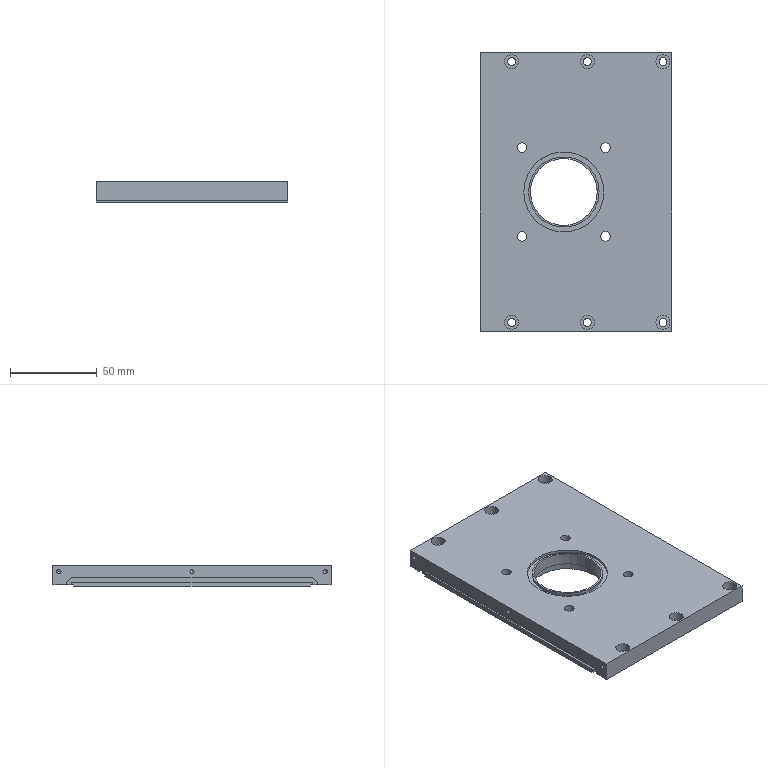NC program | NX | posted with a generic post | part box 110 x 160 x 12 mm
Whole program:
N10 G17 G21 G94 G90
(HOLE_MILLING_1 , TOOL : D4)
N12 T11 M6
N14 G54
N16 G17 G0 G90 X-75. Y37. B0. C0. S9500 M3
N18 G43 Z30. H11
N20 Z0.5
N22 G94 G3 X-76. Y36. R1. F1650.
N24 X-75. Y35. R1.
N26 X-75. Y35. Z0.1 I0. J2.
N28 X-75. Y35. Z-0.3 I0. J2.
N30 X-75. Y35. Z-0.7 I0. J2.
N32 X-75. Y35. Z-1.1 I0. J2.
N34 X-75. Y35. Z-1.5 I0. J2.
N36 X-75. Y35. Z-1.9 I0. J2.
N38 X-75. Y35. Z-2.3 I0. J2.
N40 X-75. Y35. Z-2.7 I0. J2.
N42 X-75. Y35. Z-3.1 I0. J2.
N44 X-75. Y35. Z-3.5 I0. J2.
N46 X-75. Y35. Z-3.9 I0. J2.
N48 X-75. Y35. Z-4.3 I0. J2.
N50 X-75. Y35. Z-4.7 I0. J2.
N52 X-77. Y37. Z-5. R-2.
N54 X-75. Y35. R2.
N56 X-77. Y37. R-2.
N58 X-76. Y36. R1.
N60 X-75. Y37. R1.
N62 G0 Z30.
N64 Y-6.5
N66 Z0.5
N68 G3 X-76. Y-7.5 R1.
N70 X-75. Y-8.5 R1.
N72 X-75. Y-8.5 Z0.1 I0. J2.
N74 X-75. Y-8.5 Z-0.3 I0. J2.
N76 X-75. Y-8.5 Z-0.7 I0. J2.
N78 X-75. Y-8.5 Z-1.1 I0. J2.
N80 X-75. Y-8.5 Z-1.5 I0. J2.
N82 X-75. Y-8.5 Z-1.9 I0. J2.
N84 X-75. Y-8.5 Z-2.3 I0. J2.
N86 X-75. Y-8.5 Z-2.7 I0. J2.
N88 X-75. Y-8.5 Z-3.1 I0. J2.
N90 X-75. Y-8.5 Z-3.5 I0. J2.
N92 X-75. Y-8.5 Z-3.9 I0. J2.
N94 X-75. Y-8.5 Z-4.3 I0. J2.
N96 X-75. Y-8.5 Z-4.7 I0. J2.
N98 X-77. Y-6.5 Z-5. R-2.
N100 X-75. Y-8.5 R2.
N102 X-77. Y-6.5 R-2.
N104 X-76. Y-7.5 R1.
N106 X-75. Y-6.5 R1.
N108 G0 Z30.
N110 Y-50.
N112 Z0.5
N114 G3 X-76. Y-51. R1.
N116 X-75. Y-52. R1.
N118 X-75. Y-52. Z0.1 I0. J2.
N120 X-75. Y-52. Z-0.3 I0. J2.
N122 X-75. Y-52. Z-0.7 I0. J2.
N124 X-75. Y-52. Z-1.1 I0. J2.
N126 X-75. Y-52. Z-1.5 I0. J2.
N128 X-75. Y-52. Z-1.9 I0. J2.
N130 X-75. Y-52. Z-2.3 I0. J2.
N132 X-75. Y-52. Z-2.7 I0. J2.
N134 X-75. Y-52. Z-3.1 I0. J2.
N136 X-75. Y-52. Z-3.5 I0. J2.
N138 X-75. Y-52. Z-3.9 I0. J2.
N140 X-75. Y-52. Z-4.3 I0. J2.
N142 X-75. Y-52. Z-4.7 I0. J2.
N144 X-77. Y-50. Z-5. R-2.
N146 X-75. Y-52. R2.
N148 X-77. Y-50. R-2.
N150 X-76. Y-51. R1.
N152 X-75. Y-50. R1.
N154 G0 Z30.
N156 X75.
N158 Z0.5
N160 G3 X74. Y-51. R1.
N162 X75. Y-52. R1.
N164 X75. Y-52. Z0.1 I0. J2.
N166 X75. Y-52. Z-0.3 I0. J2.
N168 X75. Y-52. Z-0.7 I0. J2.
N170 X75. Y-52. Z-1.1 I0. J2.
N172 X75. Y-52. Z-1.5 I0. J2.
N174 X75. Y-52. Z-1.9 I0. J2.
N176 X75. Y-52. Z-2.3 I0. J2.
N178 X75. Y-52. Z-2.7 I0. J2.
N180 X75. Y-52. Z-3.1 I0. J2.
N182 X75. Y-52. Z-3.5 I0. J2.
N184 X75. Y-52. Z-3.9 I0. J2.
N186 X75. Y-52. Z-4.3 I0. J2.
N188 X75. Y-52. Z-4.7 I0. J2.
N190 X73. Y-50. Z-5. R-2.
N192 X75. Y-52. R2.
N194 X73. Y-50. R-2.
N196 X74. Y-51. R1.
N198 X75. Y-50. R1.
N200 G0 Z30.
N202 Y-6.5
N204 Z0.5
N206 G3 X74. Y-7.5 R1.
N208 X75. Y-8.5 R1.
N210 X75. Y-8.5 Z0.1 I0. J2.
N212 X75. Y-8.5 Z-0.3 I0. J2.
N214 X75. Y-8.5 Z-0.7 I0. J2.
N216 X75. Y-8.5 Z-1.1 I0. J2.
N218 X75. Y-8.5 Z-1.5 I0. J2.
N220 X75. Y-8.5 Z-1.9 I0. J2.
N222 X75. Y-8.5 Z-2.3 I0. J2.
N224 X75. Y-8.5 Z-2.7 I0. J2.
N226 X75. Y-8.5 Z-3.1 I0. J2.
N228 X75. Y-8.5 Z-3.5 I0. J2.
N230 X75. Y-8.5 Z-3.9 I0. J2.
N232 X75. Y-8.5 Z-4.3 I0. J2.
N234 X75. Y-8.5 Z-4.7 I0. J2.
N236 X73. Y-6.5 Z-5. R-2.
N238 X75. Y-8.5 R2.
N240 X73. Y-6.5 R-2.
N242 X74. Y-7.5 R1.
N244 X75. Y-6.5 R1.
N246 G0 Z30.
N248 Y37.
N250 Z0.5
N252 G3 X74. Y36. R1.
N254 X75. Y35. R1.
N256 X75. Y35. Z0.1 I0. J2.
N258 X75. Y35. Z-0.3 I0. J2.
N260 X75. Y35. Z-0.7 I0. J2.
N262 X75. Y35. Z-1.1 I0. J2.
N264 X75. Y35. Z-1.5 I0. J2.
N266 X75. Y35. Z-1.9 I0. J2.
N268 X75. Y35. Z-2.3 I0. J2.
N270 X75. Y35. Z-2.7 I0. J2.
N272 X75. Y35. Z-3.1 I0. J2.
N274 X75. Y35. Z-3.5 I0. J2.
N276 X75. Y35. Z-3.9 I0. J2.
N278 X75. Y35. Z-4.3 I0. J2.
N280 X75. Y35. Z-4.7 I0. J2.
N282 X73. Y37. Z-5. R-2.
N284 X75. Y35. R2.
N286 X73. Y37. R-2.
N288 X74. Y36. R1.
N290 X75. Y37. R1.
N292 G0 Z30.
N294 M5
(ZLEVEL_PROFILE , TOOL : D2)
N296 T02 M6
N298 G54
N300 G17 G0 G90 X19.994 Y-2.325 B0. C0. S9500 M3
N302 G43 Z30. H2
N304 Z1.
N306 G94 G1 X20.195 Y-1.926 Z0.977 F1100.
N308 X21.236 Y0.952 Z0.816
N310 X21.868 Y3.947 Z0.656
N312 X22.08 Y7. Z0.495
N314 X21.868 Y10.053 Z0.335
N316 X21.236 Y13.048 Z0.175
N318 X20.195 Y15.926 Z0.014
N320 X19.676 Y16.953 Z-0.046
N322 X19.653 Y16.999 Z-0.049
N324 X19.215 Y17.859 Z-0.099
N326 X18.703 Y18.678 Z-0.15
N328 G3 X-19.653 Y16.999 R22.05
N330 G1 X-19.676 Y16.953
N332 G3 X-9.953 Y-12.676 R22.05
N334 X19.653 Y-2.999 R22.05
N336 G1 X19.676 Y-2.953
N338 G3 X19.676 Y16.953 R22.05
N340 G1 X19.653 Y16.999
N342 G3 X18.703 Y18.678 R22.05
N344 G1 X18.604 Y18.819 Z-0.153
N346 X18.506 Y18.96 Z-0.156
N348 X18.408 Y19.101 Z-0.159
N350 X18.31 Y19.242 Z-0.162
N352 X18.212 Y19.383 Z-0.165
N354 X18.114 Y19.524 Z-0.168
N356 X18.016 Y19.665 Z-0.171
N358 X17.917 Y19.806 Z-0.174
N360 X17.819 Y19.947 Z-0.177
N362 X17.722 Y20.088 Z-0.18
N364 X17.623 Y20.229 Z-0.183
N366 X17.525 Y20.37 Z-0.186
N368 X17.426 Y20.51 Z-0.189
N370 X17.314 Y20.64 Z-0.192
N372 X17.201 Y20.771 Z-0.195
N374 X17.089 Y20.901 Z-0.198
N376 X16.978 Y21.031 Z-0.201
N378 X16.866 Y21.162 Z-0.204
N380 X16.754 Y21.292 Z-0.207
N382 X16.642 Y21.422 Z-0.21
N384 X16.53 Y21.552 Z-0.213
N386 X16.418 Y21.682 Z-0.216
N388 X16.306 Y21.813 Z-0.219
N390 X16.195 Y21.943 Z-0.222
N392 X16.082 Y22.074 Z-0.225
N394 X15.97 Y22.204 Z-0.228
N396 X15.845 Y22.322 Z-0.231
N398 X15.72 Y22.44 Z-0.234
N400 X15.595 Y22.558 Z-0.237
N402 X15.471 Y22.677 Z-0.24
N404 X15.346 Y22.795 Z-0.243
N406 X15.222 Y22.913 Z-0.246
N408 X15.098 Y23.031 Z-0.249
N410 X14.973 Y23.15 Z-0.252
N412 X14.849 Y23.268 Z-0.255
N414 X14.725 Y23.387 Z-0.258
N416 X14.6 Y23.505 Z-0.261
N418 X14.475 Y23.623 Z-0.264
N420 X14.35 Y23.741 Z-0.267
N422 X14.214 Y23.846 Z-0.27
N424 X14.078 Y23.951 Z-0.273
N426 X13.942 Y24.056 Z-0.276
N428 X13.806 Y24.161 Z-0.279
N430 X13.67 Y24.267 Z-0.282
N432 X13.534 Y24.371 Z-0.285
N434 X13.399 Y24.476 Z-0.288
N436 X13.263 Y24.581 Z-0.291
N438 X13.127 Y24.686 Z-0.294
N440 X12.991 Y24.792 Z-0.297
N442 X12.864 Y24.909 Z-0.3
N444 G3 X-19.653 Y16.999 R22.05
N446 G1 X-19.676 Y16.953
N448 G3 X-9.953 Y-12.676 R22.05
N450 X19.653 Y-2.999 R22.05
N452 G1 X19.676 Y-2.953
N454 G3 X19.676 Y16.953 R22.05
N456 G1 X19.653 Y16.999
N458 G3 X18.703 Y18.678 R22.05
N460 G1 X18.605 Y18.819 Z-0.303
N462 X18.506 Y18.96 Z-0.306
N464 X18.408 Y19.101 Z-0.309
N466 X18.31 Y19.242 Z-0.312
N468 X18.211 Y19.383 Z-0.315
N470 X18.114 Y19.524 Z-0.318
N472 X18.015 Y19.664 Z-0.321
N474 X17.917 Y19.805 Z-0.324
N476 X17.819 Y19.946 Z-0.327
N478 X17.722 Y20.088 Z-0.33
N480 X17.623 Y20.228 Z-0.333
N482 X17.525 Y20.37 Z-0.336
N484 X17.426 Y20.51 Z-0.339
N486 X17.313 Y20.64 Z-0.342
N488 X17.201 Y20.77 Z-0.345
N490 X17.089 Y20.901 Z-0.348
N492 X16.977 Y21.031 Z-0.351
N494 X16.866 Y21.162 Z-0.354
N496 X16.754 Y21.292 Z-0.357
N498 X16.642 Y21.422 Z-0.36
N500 X16.53 Y21.552 Z-0.363
N502 X16.418 Y21.682 Z-0.366
N504 X16.306 Y21.813 Z-0.369
N506 X16.195 Y21.943 Z-0.372
N508 X16.083 Y22.074 Z-0.375
N510 X15.97 Y22.204 Z-0.378
N512 X15.845 Y22.322 Z-0.381
N514 X15.72 Y22.44 Z-0.384
N516 X15.596 Y22.559 Z-0.387
N518 X15.471 Y22.676 Z-0.39
N520 X15.347 Y22.795 Z-0.393
N522 X15.222 Y22.913 Z-0.396
N524 X15.097 Y23.031 Z-0.399
N526 X14.973 Y23.15 Z-0.402
N528 X14.849 Y23.268 Z-0.405
N530 X14.725 Y23.387 Z-0.408
N532 X14.6 Y23.505 Z-0.411
N534 X14.475 Y23.623 Z-0.414
N536 X14.35 Y23.741 Z-0.417
N538 X14.214 Y23.846 Z-0.42
N540 X14.077 Y23.951 Z-0.423
N542 X13.942 Y24.056 Z-0.426
N544 X13.806 Y24.161 Z-0.429
N546 X13.67 Y24.266 Z-0.432
N548 X13.534 Y24.371 Z-0.435
N550 X13.399 Y24.476 Z-0.438
N552 X13.263 Y24.582 Z-0.441
N554 X13.127 Y24.686 Z-0.444
N556 X12.991 Y24.792 Z-0.447
N558 X12.864 Y24.909 Z-0.45
N560 G3 X-19.653 Y16.999 R22.05
N562 G1 X-19.676 Y16.953
N564 G3 X-9.953 Y-12.676 R22.05
N566 X19.653 Y-2.999 R22.05
N568 G1 X19.676 Y-2.953
N570 G3 X19.676 Y16.953 R22.05
N572 G1 X19.653 Y16.999
N574 G3 X18.703 Y18.678 R22.05
N576 G1 X18.604 Y18.819 Z-0.453
N578 X18.506 Y18.96 Z-0.456
N580 X18.408 Y19.101 Z-0.459
N582 X18.309 Y19.242 Z-0.462
N584 X18.212 Y19.383 Z-0.465
N586 X18.114 Y19.524 Z-0.468
N588 X18.016 Y19.665 Z-0.471
N590 X17.917 Y19.805 Z-0.474
N592 X17.819 Y19.946 Z-0.477
N594 X17.721 Y20.087 Z-0.48
N596 X17.623 Y20.228 Z-0.483
N598 X17.525 Y20.37 Z-0.486
N600 X17.426 Y20.51 Z-0.489
N602 X17.313 Y20.64 Z-0.492
N604 X17.201 Y20.77 Z-0.495
N606 X17.089 Y20.901 Z-0.498
N608 X16.978 Y21.031 Z-0.501
N610 X16.866 Y21.162 Z-0.504
N612 X16.753 Y21.291 Z-0.507
N614 X16.642 Y21.422 Z-0.51
N616 X16.53 Y21.552 Z-0.513
N618 X16.418 Y21.682 Z-0.516
N620 X16.307 Y21.813 Z-0.519
N622 X16.195 Y21.943 Z-0.522
N624 X16.083 Y22.074 Z-0.525
N626 X15.97 Y22.204 Z-0.528
N628 X15.845 Y22.321 Z-0.531
N630 X15.72 Y22.44 Z-0.534
N632 X15.595 Y22.558 Z-0.537
N634 X15.471 Y22.676 Z-0.54
N636 X15.347 Y22.795 Z-0.543
N638 X15.222 Y22.913 Z-0.546
N640 X15.098 Y23.031 Z-0.549
N642 X14.973 Y23.149 Z-0.552
N644 X14.849 Y23.268 Z-0.555
N646 X14.724 Y23.386 Z-0.558
N648 X14.599 Y23.504 Z-0.561
N650 X14.475 Y23.623 Z-0.564
N652 X14.35 Y23.741 Z-0.567
N654 X14.213 Y23.846 Z-0.57
N656 X14.078 Y23.951 Z-0.573
N658 X13.941 Y24.056 Z-0.576
N660 X13.806 Y24.161 Z-0.579
N662 X13.67 Y24.266 Z-0.582
N664 X13.534 Y24.371 Z-0.585
N666 X13.398 Y24.476 Z-0.588
N668 X13.263 Y24.581 Z-0.591
N670 X13.127 Y24.686 Z-0.594
N672 X12.991 Y24.791 Z-0.597
N674 X12.864 Y24.909 Z-0.6
N676 G3 X-19.653 Y16.999 R22.05
N678 G1 X-19.676 Y16.953
N680 G3 X-9.953 Y-12.676 R22.05
N682 X19.653 Y-2.999 R22.05
N684 G1 X19.676 Y-2.953
N686 G3 X19.676 Y16.953 R22.05
N688 G1 X19.653 Y16.999
N690 G3 X18.703 Y18.678 R22.05
N692 G1 X18.604 Y18.819 Z-0.603
N694 X18.506 Y18.96 Z-0.606
N696 X18.408 Y19.101 Z-0.609
N698 X18.309 Y19.242 Z-0.612
N700 X18.211 Y19.383 Z-0.615
N702 X18.113 Y19.524 Z-0.618
N704 X18.015 Y19.665 Z-0.621
N706 X17.917 Y19.805 Z-0.624
N708 X17.819 Y19.946 Z-0.627
N710 X17.721 Y20.087 Z-0.63
N712 X17.622 Y20.228 Z-0.633
N714 X17.525 Y20.369 Z-0.636
N716 X17.426 Y20.51 Z-0.639
N718 X17.313 Y20.64 Z-0.642
N720 X17.201 Y20.77 Z-0.645
N722 X17.089 Y20.901 Z-0.648
N724 X16.977 Y21.031 Z-0.651
N726 X16.866 Y21.161 Z-0.654
N728 X16.754 Y21.292 Z-0.657
N730 X16.642 Y21.422 Z-0.66
N732 X16.53 Y21.552 Z-0.663
N734 X16.418 Y21.682 Z-0.666
N736 X16.306 Y21.813 Z-0.669
N738 X16.194 Y21.943 Z-0.672
N740 X16.082 Y22.074 Z-0.675
N742 X15.97 Y22.204 Z-0.678
N744 X15.844 Y22.321 Z-0.681
N746 X15.72 Y22.44 Z-0.684
N748 X15.595 Y22.558 Z-0.687
N750 X15.471 Y22.676 Z-0.69
N752 X15.346 Y22.795 Z-0.693
N754 X15.222 Y22.913 Z-0.696
N756 X15.098 Y23.031 Z-0.699
N758 X14.973 Y23.149 Z-0.702
N760 X14.849 Y23.268 Z-0.705
N762 X14.724 Y23.386 Z-0.708
N764 X14.6 Y23.505 Z-0.711
N766 X14.475 Y23.623 Z-0.714
N768 X14.35 Y23.741 Z-0.717
N770 X14.213 Y23.846 Z-0.72
N772 X14.077 Y23.951 Z-0.723
N774 X13.941 Y24.056 Z-0.726
N776 X13.806 Y24.161 Z-0.729
N778 X13.67 Y24.266 Z-0.732
N780 X13.534 Y24.371 Z-0.735
N782 X13.398 Y24.476 Z-0.738
N784 X13.263 Y24.581 Z-0.741
N786 X13.127 Y24.686 Z-0.744
N788 X12.991 Y24.791 Z-0.747
N790 X12.864 Y24.909 Z-0.75
N792 G3 X-19.653 Y16.999 R22.05
N794 G1 X-19.676 Y16.953
N796 G3 X-9.953 Y-12.676 R22.05
N798 X19.653 Y-2.999 R22.05
N800 G1 X19.676 Y-2.953
N802 G3 X19.676 Y16.953 R22.05
N804 G1 X19.653 Y16.999
N806 G3 X18.703 Y18.678 R22.05
N808 G1 X18.604 Y18.819 Z-0.753
N810 X18.506 Y18.96 Z-0.756
N812 X18.407 Y19.101 Z-0.759
N814 X18.309 Y19.242 Z-0.762
N816 X18.211 Y19.382 Z-0.765
N818 X18.113 Y19.523 Z-0.768
N820 X18.015 Y19.664 Z-0.771
N822 X17.917 Y19.805 Z-0.774
N824 X17.819 Y19.946 Z-0.777
N826 X17.721 Y20.087 Z-0.78
N828 X17.623 Y20.228 Z-0.783
N830 X17.525 Y20.369 Z-0.786
N832 X17.426 Y20.51 Z-0.789
N834 X17.313 Y20.64 Z-0.792
N836 X17.201 Y20.77 Z-0.795
N838 X17.089 Y20.901 Z-0.798
N840 X16.977 Y21.031 Z-0.801
N842 X16.865 Y21.161 Z-0.804
N844 X16.753 Y21.291 Z-0.807
N846 X16.642 Y21.422 Z-0.81
N848 X16.53 Y21.552 Z-0.813
N850 X16.418 Y21.682 Z-0.816
N852 X16.306 Y21.812 Z-0.819
N854 X16.194 Y21.943 Z-0.822
N856 X16.082 Y22.073 Z-0.825
N858 X15.97 Y22.204 Z-0.828
N860 X15.844 Y22.321 Z-0.831
N862 X15.72 Y22.44 Z-0.834
N864 X15.595 Y22.558 Z-0.837
N866 X15.47 Y22.676 Z-0.84
N868 X15.346 Y22.794 Z-0.843
N870 X15.222 Y22.913 Z-0.846
N872 X15.097 Y23.031 Z-0.849
N874 X14.973 Y23.149 Z-0.852
N876 X14.848 Y23.268 Z-0.855
N878 X14.724 Y23.386 Z-0.858
N880 X14.6 Y23.504 Z-0.861
N882 X14.475 Y23.623 Z-0.864
N884 X14.35 Y23.741 Z-0.867
N886 X14.213 Y23.845 Z-0.87
N888 X14.077 Y23.95 Z-0.873
N890 X13.941 Y24.056 Z-0.876
N892 X13.805 Y24.161 Z-0.879
N894 X13.67 Y24.266 Z-0.882
N896 X13.534 Y24.371 Z-0.885
N898 X13.398 Y24.476 Z-0.888
N900 X13.262 Y24.581 Z-0.891
N902 X13.127 Y24.686 Z-0.894
N904 X12.991 Y24.791 Z-0.897
N906 X12.864 Y24.909 Z-0.9
N908 G3 X-19.653 Y16.999 R22.05
N910 G1 X-19.676 Y16.953
N912 G3 X-9.953 Y-12.676 R22.05
N914 X19.653 Y-2.999 R22.05
N916 G1 X19.676 Y-2.953
N918 G3 X19.676 Y16.953 R22.05
N920 G1 X19.653 Y16.999
N922 G3 X18.703 Y18.678 R22.05
N924 G1 X18.604 Y18.818 Z-0.903
N926 X18.506 Y18.96 Z-0.906
N928 X18.407 Y19.1 Z-0.909
N930 X18.309 Y19.241 Z-0.912
N932 X18.211 Y19.382 Z-0.915
N934 X18.113 Y19.523 Z-0.918
N936 X18.015 Y19.664 Z-0.921
N938 X17.917 Y19.805 Z-0.924
N940 X17.819 Y19.946 Z-0.927
N942 X17.721 Y20.087 Z-0.93
N944 X17.623 Y20.228 Z-0.933
N946 X17.524 Y20.369 Z-0.936
N948 X17.426 Y20.51 Z-0.939
N950 X17.313 Y20.64 Z-0.942
N952 X17.201 Y20.77 Z-0.945
N954 X17.089 Y20.9 Z-0.948
N956 X16.977 Y21.031 Z-0.951
N958 X16.865 Y21.161 Z-0.954
N960 X16.753 Y21.291 Z-0.957
N962 X16.641 Y21.422 Z-0.96
N964 X16.529 Y21.552 Z-0.963
N966 X16.418 Y21.682 Z-0.966
N968 X16.306 Y21.812 Z-0.969
N970 X16.194 Y21.943 Z-0.972
N972 X16.082 Y22.073 Z-0.975
N974 X15.97 Y22.204 Z-0.978
N976 X15.844 Y22.321 Z-0.981
N978 X15.72 Y22.44 Z-0.984
N980 X15.595 Y22.558 Z-0.987
N982 X15.47 Y22.676 Z-0.99
N984 X15.346 Y22.794 Z-0.993
N986 X15.222 Y22.913 Z-0.996
N988 X15.097 Y23.031 Z-0.999
N990 X14.973 Y23.149 Z-1.002
N992 X14.848 Y23.267 Z-1.005
N994 X14.724 Y23.386 Z-1.008
N996 X14.599 Y23.504 Z-1.011
N998 X14.475 Y23.623 Z-1.014
N1000 X14.35 Y23.741 Z-1.017
N1002 X14.213 Y23.845 Z-1.02
N1004 X14.077 Y23.95 Z-1.023
N1006 X13.941 Y24.055 Z-1.026
N1008 X13.805 Y24.16 Z-1.029
N1010 X13.67 Y24.266 Z-1.032
N1012 X13.534 Y24.371 Z-1.035
N1014 X13.398 Y24.476 Z-1.038
N1016 X13.262 Y24.581 Z-1.041
N1018 X13.127 Y24.686 Z-1.044
N1020 X12.991 Y24.791 Z-1.047
N1022 X12.864 Y24.909 Z-1.05
N1024 G3 X-19.653 Y16.999 R22.05
N1026 G1 X-19.676 Y16.953
N1028 G3 X-9.953 Y-12.676 R22.05
N1030 X19.653 Y-2.999 R22.05
N1032 G1 X19.676 Y-2.953
N1034 G3 X19.676 Y16.953 R22.05
N1036 G1 X19.653 Y16.999
N1038 G3 X18.703 Y18.678 R22.05
N1040 G1 X18.603 Y18.818 Z-1.053
N1042 X18.505 Y18.96 Z-1.056
N1044 X18.407 Y19.1 Z-1.059
N1046 X18.309 Y19.241 Z-1.062
N1048 X18.211 Y19.382 Z-1.065
N1050 X18.113 Y19.523 Z-1.068
N1052 X18.015 Y19.664 Z-1.071
N1054 X17.917 Y19.805 Z-1.074
N1056 X17.818 Y19.946 Z-1.077
N1058 X17.721 Y20.087 Z-1.08
N1060 X17.622 Y20.228 Z-1.083
N1062 X17.524 Y20.369 Z-1.086
N1064 X17.426 Y20.51 Z-1.089
N1066 X17.313 Y20.64 Z-1.092
N1068 X17.2 Y20.77 Z-1.095
N1070 X17.089 Y20.9 Z-1.098
N1072 X16.977 Y21.03 Z-1.101
N1074 X16.865 Y21.161 Z-1.104
N1076 X16.753 Y21.291 Z-1.107
N1078 X16.641 Y21.421 Z-1.11
N1080 X16.53 Y21.552 Z-1.113
N1082 X16.418 Y21.682 Z-1.116
N1084 X16.306 Y21.812 Z-1.119
N1086 X16.194 Y21.943 Z-1.122
N1088 X16.082 Y22.073 Z-1.125
N1090 X15.97 Y22.204 Z-1.128
N1092 X15.844 Y22.321 Z-1.131
N1094 X15.719 Y22.439 Z-1.134
N1096 X15.595 Y22.558 Z-1.137
N1098 X15.47 Y22.676 Z-1.14
N1100 X15.346 Y22.795 Z-1.143
N1102 X15.222 Y22.913 Z-1.146
N1104 X15.097 Y23.031 Z-1.149
N1106 X14.973 Y23.149 Z-1.152
N1108 X14.848 Y23.267 Z-1.155
N1110 X14.724 Y23.386 Z-1.158
N1112 X14.599 Y23.504 Z-1.161
N1114 X14.475 Y23.623 Z-1.164
N1116 X14.35 Y23.741 Z-1.167
N1118 X14.213 Y23.845 Z-1.17
N1120 X14.077 Y23.95 Z-1.173
N1122 X13.941 Y24.055 Z-1.176
N1124 X13.805 Y24.16 Z-1.179
N1126 X13.67 Y24.266 Z-1.182
N1128 X13.534 Y24.37 Z-1.185
N1130 X13.398 Y24.476 Z-1.188
N1132 X13.262 Y24.581 Z-1.191
N1134 X13.126 Y24.686 Z-1.194
N1136 X12.991 Y24.791 Z-1.197
N1138 X12.864 Y24.909 Z-1.2
N1140 G3 X-19.653 Y16.999 R22.05
N1142 G1 X-19.676 Y16.953
N1144 G3 X-9.953 Y-12.676 R22.05
N1146 X19.653 Y-2.999 R22.05
N1148 G1 X19.676 Y-2.953
N1150 G3 X19.676 Y16.953 R22.05
N1152 G1 X19.653 Y16.999
N1154 G3 X18.703 Y18.678 R22.05
N1156 G1 X18.603 Y18.818 Z-1.203
N1158 X18.505 Y18.959 Z-1.206
N1160 X18.407 Y19.101 Z-1.209
N1162 X18.309 Y19.241 Z-1.212
N1164 X18.211 Y19.382 Z-1.215
N1166 X18.113 Y19.523 Z-1.218
N1168 X18.015 Y19.664 Z-1.221
N1170 X17.917 Y19.805 Z-1.224
N1172 X17.818 Y19.946 Z-1.227
N1174 X17.721 Y20.087 Z-1.23
N1176 X17.622 Y20.228 Z-1.233
N1178 X17.524 Y20.369 Z-1.236
N1180 X17.426 Y20.51 Z-1.239
N1182 X17.313 Y20.64 Z-1.242
N1184 X17.2 Y20.77 Z-1.245
N1186 X17.088 Y20.9 Z-1.248
N1188 X16.977 Y21.031 Z-1.251
N1190 X16.865 Y21.161 Z-1.254
N1192 X16.753 Y21.291 Z-1.257
N1194 X16.641 Y21.421 Z-1.26
N1196 X16.529 Y21.552 Z-1.263
N1198 X16.417 Y21.682 Z-1.266
N1200 X16.306 Y21.812 Z-1.269
N1202 X16.194 Y21.943 Z-1.272
N1204 X16.082 Y22.073 Z-1.275
N1206 X15.97 Y22.204 Z-1.278
N1208 X15.844 Y22.321 Z-1.281
N1210 X15.719 Y22.439 Z-1.284
N1212 X15.595 Y22.558 Z-1.287
N1214 X15.47 Y22.676 Z-1.29
N1216 X15.346 Y22.794 Z-1.293
N1218 X15.221 Y22.912 Z-1.296
N1220 X15.097 Y23.031 Z-1.299
N1222 X14.973 Y23.149 Z-1.302
N1224 X14.848 Y23.267 Z-1.305
N1226 X14.724 Y23.386 Z-1.308
N1228 X14.599 Y23.504 Z-1.311
N1230 X14.475 Y23.622 Z-1.314
N1232 X14.35 Y23.741 Z-1.317
N1234 X14.213 Y23.845 Z-1.32
N1236 X14.077 Y23.95 Z-1.323
N1238 X13.941 Y24.055 Z-1.326
N1240 X13.805 Y24.161 Z-1.329
N1242 X13.67 Y24.266 Z-1.332
N1244 X13.534 Y24.371 Z-1.335
N1246 X13.398 Y24.476 Z-1.338
N1248 X13.262 Y24.581 Z-1.341
N1250 X13.126 Y24.686 Z-1.344
N1252 X12.991 Y24.791 Z-1.347
N1254 X12.864 Y24.909 Z-1.35
N1256 G3 X-19.653 Y16.999 R22.05
N1258 G1 X-19.676 Y16.953
N1260 G3 X-9.953 Y-12.676 R22.05
N1262 X19.653 Y-2.999 R22.05
N1264 G1 X19.676 Y-2.953
N1266 G3 X19.676 Y16.953 R22.05
N1268 G1 X19.653 Y16.999
N1270 G3 X18.703 Y18.678 R22.05
N1272 G1 X18.603 Y18.818 Z-1.353
N1274 X18.505 Y18.959 Z-1.356
N1276 X18.407 Y19.1 Z-1.359
N1278 X18.309 Y19.241 Z-1.362
N1280 X18.211 Y19.382 Z-1.365
N1282 X18.113 Y19.523 Z-1.368
N1284 X18.015 Y19.664 Z-1.371
N1286 X17.916 Y19.805 Z-1.374
N1288 X17.819 Y19.946 Z-1.377
N1290 X17.721 Y20.087 Z-1.38
N1292 X17.622 Y20.227 Z-1.383
N1294 X17.524 Y20.369 Z-1.386
N1296 X17.426 Y20.51 Z-1.389
N1298 X17.312 Y20.64 Z-1.392
N1300 X17.2 Y20.77 Z-1.395
N1302 X17.088 Y20.9 Z-1.398
N1304 X16.977 Y21.031 Z-1.401
N1306 X16.865 Y21.161 Z-1.404
N1308 X16.753 Y21.291 Z-1.407
N1310 X16.641 Y21.421 Z-1.41
N1312 X16.529 Y21.551 Z-1.413
N1314 X16.417 Y21.682 Z-1.416
N1316 X16.306 Y21.812 Z-1.419
N1318 X16.194 Y21.943 Z-1.422
N1320 X16.081 Y22.073 Z-1.425
N1322 X15.97 Y22.204 Z-1.428
N1324 X15.844 Y22.32 Z-1.431
N1326 X15.719 Y22.439 Z-1.434
N1328 X15.595 Y22.557 Z-1.437
N1330 X15.47 Y22.676 Z-1.44
N1332 X15.346 Y22.794 Z-1.443
N1334 X15.221 Y22.912 Z-1.446
N1336 X15.097 Y23.031 Z-1.449
N1338 X14.972 Y23.149 Z-1.452
N1340 X14.848 Y23.267 Z-1.455
N1342 X14.724 Y23.386 Z-1.458
N1344 X14.599 Y23.504 Z-1.461
N1346 X14.475 Y23.622 Z-1.464
N1348 X14.35 Y23.741 Z-1.467
N1350 X14.213 Y23.845 Z-1.47
N1352 X14.077 Y23.95 Z-1.473
N1354 X13.941 Y24.055 Z-1.476
N1356 X13.805 Y24.16 Z-1.479
N1358 X13.669 Y24.265 Z-1.482
N1360 X13.534 Y24.37 Z-1.485
N1362 X13.398 Y24.475 Z-1.488
N1364 X13.262 Y24.58 Z-1.491
N1366 X13.126 Y24.685 Z-1.494
N1368 X12.991 Y24.791 Z-1.497
N1370 X12.864 Y24.909 Z-1.5
N1372 G3 X-19.653 Y16.999 R22.05
N1374 G1 X-19.676 Y16.953
N1376 G3 X-9.953 Y-12.676 R22.05
N1378 X19.653 Y-2.999 R22.05
N1380 G1 X19.676 Y-2.953
N1382 G3 X19.676 Y16.953 R22.05
N1384 G1 X19.653 Y16.999
N1386 G3 X12.864 Y24.909 R22.05
N1388 G1 Z-0.5
N1390 G0 Z30.
N1392 X-18.252 Y17.909
N1394 Z1.
N1396 G1 X-16.601 Y20.314 Z0.847
N1398 X-14.454 Y22.618 Z0.682
N1400 X-11.992 Y24.579 Z0.517
N1402 X-10.061 Y25.752 Z0.399
N1404 X-7.217 Y27.019 Z0.236
N1406 X-4.218 Y27.858 Z0.072
N1408 X-1.13 Y28.25 Z-0.091
N1410 X0. Z-0.15
N1412 G2 X21.25 Y7. R21.25
N1414 X0. Y28.25 R-21.25
N1416 G1 X0.172 Y28.249 Z-0.153
N1418 X0.344 Y28.247 Z-0.156
N1420 X0.516 Y28.244 Z-0.159
N1422 X0.687 Y28.239 Z-0.162
N1424 X0.859 Y28.233 Z-0.165
N1426 X1.031 Y28.225 Z-0.168
N1428 X1.202 Y28.216 Z-0.171
N1430 X1.374 Y28.206 Z-0.174
N1432 X1.545 Y28.194 Z-0.177
N1434 X1.717 Y28.181 Z-0.18
N1436 X1.888 Y28.166 Z-0.183
N1438 X2.059 Y28.15 Z-0.186
N1440 X2.23 Y28.133 Z-0.189
N1442 X2.401 Y28.114 Z-0.192
N1444 X2.572 Y28.094 Z-0.195
N1446 X2.742 Y28.072 Z-0.198
N1448 X2.913 Y28.049 Z-0.201
N1450 X3.083 Y28.025 Z-0.204
N1452 X3.253 Y28. Z-0.207
N1454 X3.422 Y27.973 Z-0.21
N1456 X3.592 Y27.944 Z-0.213
N1458 X3.761 Y27.914 Z-0.216
N1460 X3.93 Y27.883 Z-0.219
N1462 X4.099 Y27.851 Z-0.222
N1464 X4.268 Y27.817 Z-0.225
N1466 X4.436 Y27.782 Z-0.228
N1468 X4.604 Y27.745 Z-0.231
N1470 X4.771 Y27.707 Z-0.234
N1472 X4.939 Y27.668 Z-0.237
N1474 X5.106 Y27.628 Z-0.24
N1476 X5.272 Y27.586 Z-0.243
N1478 X5.439 Y27.542 Z-0.246
N1480 X5.605 Y27.498 Z-0.249
N1482 X5.77 Y27.452 Z-0.252
N1484 X5.935 Y27.404 Z-0.255
N1486 X6.1 Y27.356 Z-0.258
N1488 X6.265 Y27.306 Z-0.261
N1490 X6.429 Y27.254 Z-0.264
N1492 X6.592 Y27.202 Z-0.267
N1494 X6.755 Y27.148 Z-0.27
N1496 X6.918 Y27.092 Z-0.273
N1498 X7.081 Y27.036 Z-0.276
N1500 X7.242 Y26.978 Z-0.279
N1502 X7.404 Y26.919 Z-0.282
N1504 X7.565 Y26.858 Z-0.285
N1506 X7.725 Y26.796 Z-0.288
N1508 X7.885 Y26.733 Z-0.291
N1510 X8.044 Y26.669 Z-0.294
N1512 X8.203 Y26.603 Z-0.297
N1514 X8.361 Y26.536 Z-0.3
N1516 G2 X0. Y28.25 R-21.25
N1518 G1 X0.172 Y28.249 Z-0.303
N1520 X0.344 Y28.247 Z-0.306
N1522 X0.516 Y28.244 Z-0.309
N1524 X0.687 Y28.239 Z-0.312
N1526 X0.859 Y28.233 Z-0.315
N1528 X1.031 Y28.225 Z-0.318
N1530 X1.202 Y28.216 Z-0.321
N1532 X1.374 Y28.206 Z-0.324
N1534 X1.545 Y28.194 Z-0.327
N1536 X1.717 Y28.181 Z-0.33
N1538 X1.888 Y28.166 Z-0.333
N1540 X2.059 Y28.15 Z-0.336
N1542 X2.23 Y28.133 Z-0.339
N1544 X2.401 Y28.114 Z-0.342
N1546 X2.572 Y28.094 Z-0.345
N1548 X2.742 Y28.072 Z-0.348
N1550 X2.913 Y28.049 Z-0.351
N1552 X3.083 Y28.025 Z-0.354
N1554 X3.253 Y28. Z-0.357
N1556 X3.422 Y27.973 Z-0.36
N1558 X3.592 Y27.944 Z-0.363
N1560 X3.761 Y27.914 Z-0.366
N1562 X3.93 Y27.883 Z-0.369
N1564 X4.099 Y27.851 Z-0.372
N1566 X4.268 Y27.817 Z-0.375
N1568 X4.436 Y27.782 Z-0.378
N1570 X4.604 Y27.745 Z-0.381
N1572 X4.771 Y27.707 Z-0.384
N1574 X4.939 Y27.668 Z-0.387
N1576 X5.106 Y27.628 Z-0.39
N1578 X5.272 Y27.586 Z-0.393
N1580 X5.439 Y27.542 Z-0.396
N1582 X5.605 Y27.498 Z-0.399
N1584 X5.77 Y27.452 Z-0.402
N1586 X5.935 Y27.404 Z-0.405
N1588 X6.1 Y27.356 Z-0.408
N1590 X6.265 Y27.306 Z-0.411
N1592 X6.429 Y27.254 Z-0.414
N1594 X6.592 Y27.202 Z-0.417
N1596 X6.755 Y27.148 Z-0.42
N1598 X6.918 Y27.092 Z-0.423
N1600 X7.081 Y27.036 Z-0.426
N1602 X7.242 Y26.978 Z-0.429
N1604 X7.404 Y26.919 Z-0.432
N1606 X7.565 Y26.858 Z-0.435
N1608 X7.725 Y26.796 Z-0.438
N1610 X7.885 Y26.733 Z-0.441
N1612 X8.044 Y26.669 Z-0.444
N1614 X8.203 Y26.603 Z-0.447
N1616 X8.361 Y26.536 Z-0.45
N1618 G2 X0. Y28.25 R-21.25
N1620 G1 X0.172 Y28.249 Z-0.453
N1622 X0.344 Y28.247 Z-0.456
N1624 X0.516 Y28.244 Z-0.459
N1626 X0.687 Y28.239 Z-0.462
N1628 X0.859 Y28.233 Z-0.465
N1630 X1.031 Y28.225 Z-0.468
N1632 X1.202 Y28.216 Z-0.471
N1634 X1.374 Y28.206 Z-0.474
N1636 X1.545 Y28.194 Z-0.477
N1638 X1.717 Y28.181 Z-0.48
N1640 X1.888 Y28.166 Z-0.483
N1642 X2.059 Y28.15 Z-0.486
N1644 X2.23 Y28.133 Z-0.489
N1646 X2.401 Y28.114 Z-0.492
N1648 X2.572 Y28.094 Z-0.495
N1650 X2.742 Y28.072 Z-0.498
N1652 X2.913 Y28.049 Z-0.501
N1654 X3.083 Y28.025 Z-0.504
N1656 X3.253 Y28. Z-0.507
N1658 X3.422 Y27.973 Z-0.51
N1660 X3.592 Y27.944 Z-0.513
N1662 X3.761 Y27.914 Z-0.516
N1664 X3.93 Y27.883 Z-0.519
N1666 X4.099 Y27.851 Z-0.522
N1668 X4.268 Y27.817 Z-0.525
N1670 X4.436 Y27.782 Z-0.528
N1672 X4.604 Y27.745 Z-0.531
N1674 X4.771 Y27.707 Z-0.534
N1676 X4.939 Y27.668 Z-0.537
N1678 X5.106 Y27.628 Z-0.54
N1680 X5.272 Y27.586 Z-0.543
N1682 X5.439 Y27.542 Z-0.546
N1684 X5.605 Y27.498 Z-0.549
N1686 X5.77 Y27.452 Z-0.552
N1688 X5.935 Y27.404 Z-0.555
N1690 X6.1 Y27.356 Z-0.558
N1692 X6.265 Y27.306 Z-0.561
N1694 X6.429 Y27.254 Z-0.564
N1696 X6.592 Y27.202 Z-0.567
N1698 X6.755 Y27.148 Z-0.57
N1700 X6.918 Y27.092 Z-0.573
N1702 X7.081 Y27.036 Z-0.576
N1704 X7.242 Y26.978 Z-0.579
N1706 X7.404 Y26.919 Z-0.582
N1708 X7.565 Y26.858 Z-0.585
N1710 X7.725 Y26.796 Z-0.588
N1712 X7.885 Y26.733 Z-0.591
N1714 X8.044 Y26.669 Z-0.594
N1716 X8.203 Y26.603 Z-0.597
N1718 X8.361 Y26.536 Z-0.6
N1720 G2 X0. Y28.25 R-21.25
N1722 G1 X0.172 Y28.249 Z-0.603
N1724 X0.344 Y28.247 Z-0.606
N1726 X0.516 Y28.244 Z-0.609
N1728 X0.687 Y28.239 Z-0.612
N1730 X0.859 Y28.233 Z-0.615
N1732 X1.031 Y28.225 Z-0.618
N1734 X1.202 Y28.216 Z-0.621
N1736 X1.374 Y28.206 Z-0.624
N1738 X1.545 Y28.194 Z-0.627
N1740 X1.717 Y28.181 Z-0.63
N1742 X1.888 Y28.166 Z-0.633
N1744 X2.059 Y28.15 Z-0.636
N1746 X2.23 Y28.133 Z-0.639
N1748 X2.401 Y28.114 Z-0.642
N1750 X2.572 Y28.094 Z-0.645
N1752 X2.742 Y28.072 Z-0.648
N1754 X2.913 Y28.049 Z-0.651
N1756 X3.083 Y28.025 Z-0.654
N1758 X3.253 Y28. Z-0.657
N1760 X3.422 Y27.973 Z-0.66
N1762 X3.592 Y27.944 Z-0.663
N1764 X3.761 Y27.914 Z-0.666
N1766 X3.93 Y27.883 Z-0.669
N1768 X4.099 Y27.851 Z-0.672
N1770 X4.268 Y27.817 Z-0.675
N1772 X4.436 Y27.782 Z-0.678
N1774 X4.604 Y27.745 Z-0.681
N1776 X4.771 Y27.707 Z-0.684
N1778 X4.939 Y27.668 Z-0.687
N1780 X5.106 Y27.628 Z-0.69
N1782 X5.272 Y27.586 Z-0.693
N1784 X5.439 Y27.542 Z-0.696
N1786 X5.605 Y27.498 Z-0.699
N1788 X5.77 Y27.452 Z-0.702
N1790 X5.935 Y27.404 Z-0.705
N1792 X6.1 Y27.356 Z-0.708
N1794 X6.265 Y27.306 Z-0.711
N1796 X6.429 Y27.254 Z-0.714
N1798 X6.592 Y27.202 Z-0.717
N1800 X6.755 Y27.148 Z-0.72
N1802 X6.918 Y27.092 Z-0.723
N1804 X7.081 Y27.036 Z-0.726
N1806 X7.242 Y26.978 Z-0.729
N1808 X7.404 Y26.919 Z-0.732
N1810 X7.565 Y26.858 Z-0.735
N1812 X7.725 Y26.796 Z-0.738
N1814 X7.885 Y26.733 Z-0.741
N1816 X8.044 Y26.669 Z-0.744
N1818 X8.203 Y26.603 Z-0.747
N1820 X8.361 Y26.536 Z-0.75
N1822 G2 X0. Y28.25 R-21.25
N1824 G1 X0.172 Y28.249 Z-0.753
N1826 X0.344 Y28.247 Z-0.756
N1828 X0.516 Y28.244 Z-0.759
N1830 X0.687 Y28.239 Z-0.762
N1832 X0.859 Y28.233 Z-0.765
N1834 X1.031 Y28.225 Z-0.768
N1836 X1.202 Y28.216 Z-0.771
N1838 X1.374 Y28.206 Z-0.774
N1840 X1.545 Y28.194 Z-0.777
N1842 X1.717 Y28.181 Z-0.78
N1844 X1.888 Y28.166 Z-0.783
N1846 X2.059 Y28.15 Z-0.786
N1848 X2.23 Y28.133 Z-0.789
N1850 X2.401 Y28.114 Z-0.792
N1852 X2.572 Y28.094 Z-0.795
N1854 X2.742 Y28.072 Z-0.798
N1856 X2.913 Y28.049 Z-0.801
N1858 X3.083 Y28.025 Z-0.804
N1860 X3.253 Y28. Z-0.807
N1862 X3.422 Y27.973 Z-0.81
N1864 X3.592 Y27.944 Z-0.813
N1866 X3.761 Y27.914 Z-0.816
N1868 X3.93 Y27.883 Z-0.819
N1870 X4.099 Y27.851 Z-0.822
N1872 X4.268 Y27.817 Z-0.825
N1874 X4.436 Y27.782 Z-0.828
N1876 X4.604 Y27.745 Z-0.831
N1878 X4.771 Y27.707 Z-0.834
N1880 X4.939 Y27.668 Z-0.837
N1882 X5.106 Y27.628 Z-0.84
N1884 X5.272 Y27.586 Z-0.843
N1886 X5.439 Y27.542 Z-0.846
N1888 X5.605 Y27.498 Z-0.849
N1890 X5.77 Y27.452 Z-0.852
N1892 X5.935 Y27.404 Z-0.855
N1894 X6.1 Y27.356 Z-0.858
N1896 X6.265 Y27.306 Z-0.861
N1898 X6.429 Y27.254 Z-0.864
N1900 X6.592 Y27.202 Z-0.867
N1902 X6.755 Y27.148 Z-0.87
N1904 X6.918 Y27.092 Z-0.873
N1906 X7.081 Y27.036 Z-0.876
N1908 X7.242 Y26.978 Z-0.879
N1910 X7.404 Y26.919 Z-0.882
N1912 X7.565 Y26.858 Z-0.885
N1914 X7.725 Y26.796 Z-0.888
N1916 X7.885 Y26.733 Z-0.891
N1918 X8.044 Y26.669 Z-0.894
N1920 X8.203 Y26.603 Z-0.897
N1922 X8.361 Y26.536 Z-0.9
N1924 G2 X0. Y28.25 R-21.25
N1926 G1 X0.172 Y28.249 Z-0.903
N1928 X0.344 Y28.247 Z-0.906
N1930 X0.516 Y28.244 Z-0.909
N1932 X0.687 Y28.239 Z-0.912
N1934 X0.859 Y28.233 Z-0.915
N1936 X1.031 Y28.225 Z-0.918
N1938 X1.202 Y28.216 Z-0.921
N1940 X1.374 Y28.206 Z-0.924
N1942 X1.545 Y28.194 Z-0.927
N1944 X1.717 Y28.181 Z-0.93
N1946 X1.888 Y28.166 Z-0.933
N1948 X2.059 Y28.15 Z-0.936
N1950 X2.23 Y28.133 Z-0.939
N1952 X2.401 Y28.114 Z-0.942
N1954 X2.572 Y28.094 Z-0.945
N1956 X2.742 Y28.072 Z-0.948
N1958 X2.913 Y28.049 Z-0.951
N1960 X3.083 Y28.025 Z-0.954
N1962 X3.253 Y28. Z-0.957
N1964 X3.422 Y27.973 Z-0.96
N1966 X3.592 Y27.944 Z-0.963
N1968 X3.761 Y27.914 Z-0.966
N1970 X3.93 Y27.883 Z-0.969
N1972 X4.099 Y27.851 Z-0.972
N1974 X4.268 Y27.817 Z-0.975
N1976 X4.436 Y27.782 Z-0.978
N1978 X4.604 Y27.745 Z-0.981
N1980 X4.771 Y27.707 Z-0.984
N1982 X4.939 Y27.668 Z-0.987
N1984 X5.106 Y27.628 Z-0.99
N1986 X5.272 Y27.586 Z-0.993
N1988 X5.439 Y27.542 Z-0.996
N1990 X5.605 Y27.498 Z-0.999
N1992 X5.77 Y27.452 Z-1.002
N1994 X5.935 Y27.404 Z-1.005
N1996 X6.1 Y27.356 Z-1.008
N1998 X6.265 Y27.306 Z-1.011
N2000 X6.429 Y27.254 Z-1.014
N2002 X6.592 Y27.202 Z-1.017
N2004 X6.755 Y27.148 Z-1.02
N2006 X6.918 Y27.092 Z-1.023
N2008 X7.081 Y27.036 Z-1.026
N2010 X7.242 Y26.978 Z-1.029
N2012 X7.404 Y26.919 Z-1.032
N2014 X7.565 Y26.858 Z-1.035
N2016 X7.725 Y26.796 Z-1.038
N2018 X7.885 Y26.733 Z-1.041
N2020 X8.044 Y26.669 Z-1.044
N2022 X8.203 Y26.603 Z-1.047
N2024 X8.361 Y26.536 Z-1.05
N2026 G2 X0. Y28.25 R-21.25
N2028 G1 X0.172 Y28.249 Z-1.053
N2030 X0.344 Y28.247 Z-1.056
N2032 X0.516 Y28.244 Z-1.059
N2034 X0.687 Y28.239 Z-1.062
N2036 X0.859 Y28.233 Z-1.065
N2038 X1.031 Y28.225 Z-1.068
N2040 X1.202 Y28.216 Z-1.071
N2042 X1.374 Y28.206 Z-1.074
N2044 X1.545 Y28.194 Z-1.077
N2046 X1.717 Y28.181 Z-1.08
N2048 X1.888 Y28.166 Z-1.083
N2050 X2.059 Y28.15 Z-1.086
N2052 X2.23 Y28.133 Z-1.089
N2054 X2.401 Y28.114 Z-1.092
N2056 X2.572 Y28.094 Z-1.095
N2058 X2.742 Y28.072 Z-1.098
N2060 X2.913 Y28.049 Z-1.101
N2062 X3.083 Y28.025 Z-1.104
N2064 X3.253 Y28. Z-1.107
N2066 X3.422 Y27.973 Z-1.11
N2068 X3.592 Y27.944 Z-1.113
N2070 X3.761 Y27.914 Z-1.116
N2072 X3.93 Y27.883 Z-1.119
N2074 X4.099 Y27.851 Z-1.122
N2076 X4.268 Y27.817 Z-1.125
N2078 X4.436 Y27.782 Z-1.128
N2080 X4.604 Y27.745 Z-1.131
N2082 X4.771 Y27.707 Z-1.134
N2084 X4.939 Y27.668 Z-1.137
N2086 X5.106 Y27.628 Z-1.14
N2088 X5.272 Y27.586 Z-1.143
N2090 X5.439 Y27.542 Z-1.146
N2092 X5.605 Y27.498 Z-1.149
N2094 X5.77 Y27.452 Z-1.152
N2096 X5.935 Y27.404 Z-1.155
N2098 X6.1 Y27.356 Z-1.158
N2100 X6.265 Y27.306 Z-1.161
N2102 X6.429 Y27.254 Z-1.164
N2104 X6.592 Y27.202 Z-1.167
N2106 X6.755 Y27.148 Z-1.17
N2108 X6.918 Y27.092 Z-1.173
N2110 X7.081 Y27.036 Z-1.176
N2112 X7.242 Y26.978 Z-1.179
N2114 X7.404 Y26.919 Z-1.182
N2116 X7.565 Y26.858 Z-1.185
N2118 X7.725 Y26.796 Z-1.188
N2120 X7.885 Y26.733 Z-1.191
N2122 X8.044 Y26.669 Z-1.194
N2124 X8.203 Y26.603 Z-1.197
N2126 X8.361 Y26.536 Z-1.2
N2128 G2 X0. Y28.25 R-21.25
N2130 G1 X0.172 Y28.249 Z-1.203
N2132 X0.344 Y28.247 Z-1.206
N2134 X0.516 Y28.244 Z-1.209
N2136 X0.687 Y28.239 Z-1.212
N2138 X0.859 Y28.233 Z-1.215
N2140 X1.031 Y28.225 Z-1.218
N2142 X1.202 Y28.216 Z-1.221
N2144 X1.374 Y28.206 Z-1.224
N2146 X1.545 Y28.194 Z-1.227
N2148 X1.717 Y28.181 Z-1.23
N2150 X1.888 Y28.166 Z-1.233
N2152 X2.059 Y28.15 Z-1.236
N2154 X2.23 Y28.133 Z-1.239
N2156 X2.401 Y28.114 Z-1.242
N2158 X2.572 Y28.094 Z-1.245
N2160 X2.742 Y28.072 Z-1.248
N2162 X2.913 Y28.049 Z-1.251
N2164 X3.083 Y28.025 Z-1.254
N2166 X3.253 Y28. Z-1.257
N2168 X3.422 Y27.973 Z-1.26
N2170 X3.592 Y27.944 Z-1.263
N2172 X3.761 Y27.914 Z-1.266
N2174 X3.93 Y27.883 Z-1.269
N2176 X4.099 Y27.851 Z-1.272
N2178 X4.268 Y27.817 Z-1.275
N2180 X4.436 Y27.782 Z-1.278
N2182 X4.604 Y27.745 Z-1.281
N2184 X4.771 Y27.707 Z-1.284
N2186 X4.939 Y27.668 Z-1.287
N2188 X5.106 Y27.628 Z-1.29
N2190 X5.272 Y27.586 Z-1.293
N2192 X5.439 Y27.542 Z-1.296
N2194 X5.605 Y27.498 Z-1.299
N2196 X5.77 Y27.452 Z-1.302
N2198 X5.935 Y27.404 Z-1.305
N2200 X6.1 Y27.356 Z-1.308
N2202 X6.265 Y27.306 Z-1.311
N2204 X6.429 Y27.254 Z-1.314
N2206 X6.592 Y27.202 Z-1.317
N2208 X6.755 Y27.148 Z-1.32
N2210 X6.918 Y27.092 Z-1.323
N2212 X7.081 Y27.036 Z-1.326
N2214 X7.242 Y26.978 Z-1.329
N2216 X7.404 Y26.919 Z-1.332
N2218 X7.565 Y26.858 Z-1.335
N2220 X7.725 Y26.796 Z-1.338
N2222 X7.885 Y26.733 Z-1.341
N2224 X8.044 Y26.669 Z-1.344
N2226 X8.203 Y26.603 Z-1.347
N2228 X8.361 Y26.536 Z-1.35
N2230 G2 X0. Y28.25 R-21.25
N2232 G1 X0.172 Y28.249 Z-1.353
N2234 X0.344 Y28.247 Z-1.356
N2236 X0.516 Y28.244 Z-1.359
N2238 X0.687 Y28.239 Z-1.362
N2240 X0.859 Y28.233 Z-1.365
N2242 X1.031 Y28.225 Z-1.368
N2244 X1.202 Y28.216 Z-1.371
N2246 X1.374 Y28.206 Z-1.374
N2248 X1.545 Y28.194 Z-1.377
N2250 X1.717 Y28.181 Z-1.38
N2252 X1.888 Y28.166 Z-1.383
N2254 X2.059 Y28.15 Z-1.386
N2256 X2.23 Y28.133 Z-1.389
N2258 X2.401 Y28.114 Z-1.392
N2260 X2.572 Y28.094 Z-1.395
N2262 X2.742 Y28.072 Z-1.398
N2264 X2.913 Y28.049 Z-1.401
N2266 X3.083 Y28.025 Z-1.404
N2268 X3.253 Y28. Z-1.407
N2270 X3.422 Y27.973 Z-1.41
N2272 X3.592 Y27.944 Z-1.413
N2274 X3.761 Y27.914 Z-1.416
N2276 X3.93 Y27.883 Z-1.419
N2278 X4.099 Y27.851 Z-1.422
N2280 X4.268 Y27.817 Z-1.425
N2282 X4.436 Y27.782 Z-1.428
N2284 X4.604 Y27.745 Z-1.431
N2286 X4.771 Y27.707 Z-1.434
N2288 X4.939 Y27.668 Z-1.437
N2290 X5.106 Y27.628 Z-1.44
N2292 X5.272 Y27.586 Z-1.443
N2294 X5.439 Y27.542 Z-1.446
N2296 X5.605 Y27.498 Z-1.449
N2298 X5.77 Y27.452 Z-1.452
N2300 X5.935 Y27.404 Z-1.455
N2302 X6.1 Y27.356 Z-1.458
N2304 X6.265 Y27.306 Z-1.461
N2306 X6.429 Y27.254 Z-1.464
N2308 X6.592 Y27.202 Z-1.467
N2310 X6.755 Y27.148 Z-1.47
N2312 X6.918 Y27.092 Z-1.473
N2314 X7.081 Y27.036 Z-1.476
N2316 X7.242 Y26.978 Z-1.479
N2318 X7.404 Y26.919 Z-1.482
N2320 X7.565 Y26.858 Z-1.485
N2322 X7.725 Y26.796 Z-1.488
N2324 X7.885 Y26.733 Z-1.491
N2326 X8.044 Y26.669 Z-1.494
N2328 X8.203 Y26.603 Z-1.497
N2330 X8.361 Y26.536 Z-1.5
N2332 G2 X19.536 Y-1.361 R21.25
N2334 X8.361 Y26.536 R-21.25
N2336 G1 Z-0.5
N2338 G0 Z30.
N2340 M5
(PLANAR_MILL_COPY_COPY_COPY_COPY_COPY_COPY_1_COPY_1 , TOOL : D6A45)
N2342 T01 M6
N2344 G54
N2346 G17 G0 G90 X77.94 Y-50.866 B0. C0. S9500 M3
N2348 G43 Z30. H1
N2350 Z0.84
N2352 G94 G1 Z-0.66 F1250.
N2354 G3 X78.44 Y-50. R1.
N2356 X75. Y-46.56 R3.44
N2358 X78.44 Y-50. R-3.44
N2360 X77.94 Y-49.134 R1.
N2362 G1 Z0.84
N2364 G0 Z30.
N2366 Y-7.366
N2368 Z0.84
N2370 G1 Z-0.66
N2372 G3 X78.44 Y-6.5 R1.
N2374 X75. Y-3.06 R3.44
N2376 X78.44 Y-6.5 R-3.44
N2378 X77.94 Y-5.634 R1.
N2380 G1 Z0.84
N2382 G0 Z30.
N2384 Y36.134
N2386 Z0.84
N2388 G1 Z-0.66
N2390 G3 X78.44 Y37. R1.
N2392 X75. Y40.44 R3.44
N2394 X78.44 Y37. R-3.44
N2396 X77.94 Y37.866 R1.
N2398 G1 Z0.84
N2400 G0 Z30.
N2402 X26.366 Y32.69
N2404 Z0.84
N2406 G1 Z-0.66
N2408 G3 X25.5 Y33.19 R1.
N2410 X23.31 Y31. R2.19
N2412 X25.5 Y33.19 R-2.19
N2414 X24.634 Y32.69 R1.
N2416 G1 Z0.84
N2418 G0 Z30.
N2420 X0.866 Y25.19
N2422 Z0.84
N2424 G1 Z-0.66
N2426 G3 X0. Y25.69 R1.
N2428 X-18.69 Y7. R18.69
N2430 X0. Y25.69 R-18.69
N2432 X-0.866 Y25.19 R1.
N2434 G1 Z0.84
N2436 G0 Z30.
N2438 Y28.31
N2440 Z0.84
N2442 G1 Z-0.66
N2444 G3 X0. Y27.81 R1.
N2446 G2 X20.81 Y7. R20.81
N2448 X0. Y27.81 R-20.81
N2450 G3 X0.866 Y28.31 R1.
N2452 G1 Z0.84
N2454 G0 Z30.
N2456 Y28.99
N2458 Z0.84
N2460 G1 Z-0.66
N2462 G3 X0. Y29.49 R1.
N2464 X-22.49 Y7. R22.49
N2466 X0. Y29.49 R-22.49
N2468 X-0.866 Y28.99 R1.
N2470 G1 Z0.84
N2472 G0 Z30.
N2474 X24.634 Y-18.69
N2476 Z0.84
N2478 G1 Z-0.66
N2480 G3 X25.5 Y-19.19 R1.
N2482 X27.69 Y-17. R2.19
N2484 X25.5 Y-19.19 R-2.19
N2486 X26.366 Y-18.69 R1.
N2488 G1 Z0.84
N2490 G0 Z30.
N2492 X0.866 Y-56.06
N2494 Z0.84
N2496 G1 Z-0.66
N2498 G3 X0. Y-55.56 R1.
N2500 G1 X-80.
N2502 G2 X-80.56 Y-55. R0.56
N2504 G1 Y55.
N2506 G2 X-80. Y55.56 R0.56
N2508 G1 X80.
N2510 G2 X80.56 Y55. R0.56
N2512 G1 Y-55.
N2514 G2 X80. Y-55.56 R0.56
N2516 G1 X0.
N2518 G3 X-0.866 Y-56.06 R1.
N2520 G1 Z0.84
N2522 G0 Z30.
N2524 X-26.366 Y-18.69
N2526 Z0.84
N2528 G1 Z-0.66
N2530 G3 X-25.5 Y-19.19 R1.
N2532 X-23.31 Y-17. R2.19
N2534 X-25.5 Y-19.19 R-2.19
N2536 X-24.634 Y-18.69 R1.
N2538 G1 Z0.84
N2540 G0 Z30.
N2542 Y32.69
N2544 Z0.84
N2546 G1 Z-0.66
N2548 G3 X-25.5 Y33.19 R1.
N2550 X-27.69 Y31. R2.19
N2552 X-25.5 Y33.19 R-2.19
N2554 X-26.366 Y32.69 R1.
N2556 G1 Z0.84
N2558 G0 Z30.
N2560 X-77.94 Y37.866
N2562 Z0.84
N2564 G1 Z-0.66
N2566 G3 X-78.44 Y37. R1.
N2568 X-75. Y33.56 R3.44
N2570 X-78.44 Y37. R-3.44
N2572 X-77.94 Y36.134 R1.
N2574 G1 Z0.84
N2576 G0 Z30.
N2578 Y-5.634
N2580 Z0.84
N2582 G1 Z-0.66
N2584 G3 X-78.44 Y-6.5 R1.
N2586 X-75. Y-9.94 R3.44
N2588 X-78.44 Y-6.5 R-3.44
N2590 X-77.94 Y-7.366 R1.
N2592 G1 Z0.84
N2594 G0 Z30.
N2596 Y-49.134
N2598 Z0.84
N2600 G1 Z-0.66
N2602 G3 X-78.44 Y-50. R1.
N2604 X-75. Y-53.44 R3.44
N2606 X-78.44 Y-50. R-3.44
N2608 X-77.94 Y-50.866 R1.
N2610 G1 Z0.84
N2612 G0 Z30.
N2614 M5
N2616 M2